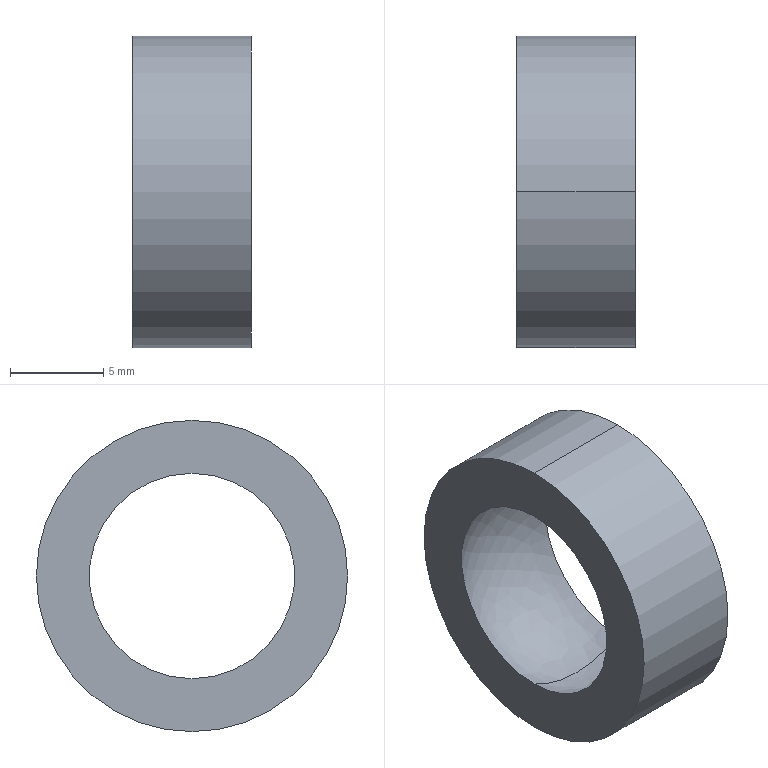Part | SolidWorks | features BaseBody 1 | 1 solid | 6 faces | box 6.35 x 16.667 x 16.667 mm | volume 648.125 mm3 | spline 2 | cylinder 2 | plane 2 | commonest cylinder face diameters 16.667 x2
STEP:
#1=CARTESIAN_POINT('',(3.175,0.,-5.499));
#2=VERTEX_POINT('',#1);
#3=CARTESIAN_POINT('',(3.175,0.,5.499));
#4=VERTEX_POINT('',#3);
#5=CARTESIAN_POINT('',(3.175,0.,0.));
#6=DIRECTION('',(1.,0.,0.));
#7=DIRECTION('',(0.,0.,1.));
#8=AXIS2_PLACEMENT_3D('',#5,#6,#7);
#9=CIRCLE('',#8,5.499);
#10=EDGE_CURVE('',#2,#4,#9,.T.);
#11=ORIENTED_EDGE('',*,*,#10,.T.);
#12=CARTESIAN_POINT('',(-3.175,0.,5.499));
#13=VERTEX_POINT('',#12);
#14=CARTESIAN_POINT('',(0.,0.,0.));
#15=DIRECTION('',(0.,-1.,0.));
#16=DIRECTION('',(1.,0.,0.));
#17=AXIS2_PLACEMENT_3D('',#14,#15,#16);
#18=CIRCLE('',#17,6.35);
#19=EDGE_CURVE('',#4,#13,#18,.T.);
#20=ORIENTED_EDGE('',*,*,#19,.T.);
#21=CARTESIAN_POINT('',(-3.175,0.,-5.499));
#22=VERTEX_POINT('',#21);
#23=CARTESIAN_POINT('',(-3.175,0.,0.));
#24=DIRECTION('',(-1.,0.,0.));
#25=DIRECTION('',(0.,0.,1.));
#26=AXIS2_PLACEMENT_3D('',#23,#24,#25);
#27=CIRCLE('',#26,5.499);
#28=EDGE_CURVE('',#13,#22,#27,.T.);
#29=ORIENTED_EDGE('',*,*,#28,.T.);
#30=CARTESIAN_POINT('',(0.,0.,0.));
#31=DIRECTION('',(0.,1.,0.));
#32=DIRECTION('',(1.,0.,0.));
#33=AXIS2_PLACEMENT_3D('',#30,#31,#32);
#34=CIRCLE('',#33,6.35);
#35=EDGE_CURVE('',#2,#22,#34,.T.);
#36=ORIENTED_EDGE('',*,*,#35,.F.);
#37=EDGE_LOOP('',(#11,#20,#29,#36));
#38=FACE_OUTER_BOUND('',#37,.T.);
#39=CARTESIAN_POINT('',(3.175,0.,5.499));
#40=CARTESIAN_POINT('',(3.175,10.999,5.499));
#41=CARTESIAN_POINT('',(3.175,10.999,-5.499));
#42=CARTESIAN_POINT('',(3.175,0.,-5.499));
#43=CARTESIAN_POINT('',(1.162,0.,6.661));
#44=CARTESIAN_POINT('',(1.162,13.323,6.661));
#45=CARTESIAN_POINT('',(1.162,13.323,-6.661));
#46=CARTESIAN_POINT('',(1.162,0.,-6.661));
#47=CARTESIAN_POINT('',(-1.162,0.,6.661));
#48=CARTESIAN_POINT('',(-1.162,13.323,6.661));
#49=CARTESIAN_POINT('',(-1.162,13.323,-6.661));
#50=CARTESIAN_POINT('',(-1.162,0.,-6.661));
#51=CARTESIAN_POINT('',(-3.175,0.,5.499));
#52=CARTESIAN_POINT('',(-3.175,10.999,5.499));
#53=CARTESIAN_POINT('',(-3.175,10.999,-5.499));
#54=CARTESIAN_POINT('',(-3.175,0.,-5.499));
#55=(BOUNDED_SURFACE()B_SPLINE_SURFACE(3,3,((#39,#40,#41,#42),(#43,#44,#45,#46),(#47,#48,#49,#50),(#51,#52,#53,#54)),.UNSPECIFIED.,.F.,.F.,.T.)B_SPLINE_SURFACE_WITH_KNOTS((4,4),(4,4),(0.,1.),(0.,1.),.UNSPECIFIED.)GEOMETRIC_REPRESENTATION_ITEM()RATIONAL_B_SPLINE_SURFACE(((1.,0.3333,0.3333,1.),(0.9107,0.3036,0.3036,0.9107),(0.9107,0.3036,0.3036,0.9107),(1.,0.3333,0.3333,1.)))REPRESENTATION_ITEM('')SURFACE());
#56=ADVANCED_FACE('',(#38),#55,.T.);
#57=CARTESIAN_POINT('',(3.175,0.,-8.334));
#58=VERTEX_POINT('',#57);
#59=CARTESIAN_POINT('',(3.175,0.,8.334));
#60=VERTEX_POINT('',#59);
#61=CARTESIAN_POINT('',(3.175,0.,0.));
#62=DIRECTION('',(1.,0.,0.));
#63=DIRECTION('',(0.,0.,1.));
#64=AXIS2_PLACEMENT_3D('',#61,#62,#63);
#65=CIRCLE('',#64,8.334);
#66=EDGE_CURVE('',#58,#60,#65,.T.);
#67=ORIENTED_EDGE('',*,*,#66,.F.);
#68=CARTESIAN_POINT('',(-3.175,0.,-8.334));
#69=VERTEX_POINT('',#68);
#70=CARTESIAN_POINT('',(3.175,0.,-8.334));
#71=DIRECTION('',(-1.,0.,0.));
#72=VECTOR('',#71,1000.);
#73=LINE('',#70,#72);
#74=EDGE_CURVE('',#58,#69,#73,.T.);
#75=ORIENTED_EDGE('',*,*,#74,.T.);
#76=CARTESIAN_POINT('',(-3.175,0.,8.334));
#77=VERTEX_POINT('',#76);
#78=CARTESIAN_POINT('',(-3.175,0.,0.));
#79=DIRECTION('',(-1.,0.,0.));
#80=DIRECTION('',(0.,0.,1.));
#81=AXIS2_PLACEMENT_3D('',#78,#79,#80);
#82=CIRCLE('',#81,8.334);
#83=EDGE_CURVE('',#77,#69,#82,.T.);
#84=ORIENTED_EDGE('',*,*,#83,.F.);
#85=CARTESIAN_POINT('',(3.175,0.,8.334));
#86=DIRECTION('',(-1.,0.,0.));
#87=VECTOR('',#86,1000.);
#88=LINE('',#85,#87);
#89=EDGE_CURVE('',#60,#77,#88,.T.);
#90=ORIENTED_EDGE('',*,*,#89,.F.);
#91=EDGE_LOOP('',(#67,#75,#84,#90));
#92=FACE_OUTER_BOUND('',#91,.T.);
#93=CARTESIAN_POINT('',(3.175,0.,0.));
#94=DIRECTION('',(-1.,0.,0.));
#95=DIRECTION('',(0.,0.,1.));
#96=AXIS2_PLACEMENT_3D('',#93,#94,#95);
#97=CYLINDRICAL_SURFACE('',#96,8.334);
#98=ADVANCED_FACE('',(#92),#97,.T.);
#99=ORIENTED_EDGE('',*,*,#19,.F.);
#100=CARTESIAN_POINT('',(3.175,0.,0.));
#101=DIRECTION('',(1.,0.,0.));
#102=DIRECTION('',(0.,0.,1.));
#103=AXIS2_PLACEMENT_3D('',#100,#101,#102);
#104=CIRCLE('',#103,5.499);
#105=EDGE_CURVE('',#4,#2,#104,.T.);
#106=ORIENTED_EDGE('',*,*,#105,.T.);
#107=ORIENTED_EDGE('',*,*,#35,.T.);
#108=CARTESIAN_POINT('',(-3.175,0.,0.));
#109=DIRECTION('',(-1.,0.,0.));
#110=DIRECTION('',(0.,0.,1.));
#111=AXIS2_PLACEMENT_3D('',#108,#109,#110);
#112=CIRCLE('',#111,5.499);
#113=EDGE_CURVE('',#22,#13,#112,.T.);
#114=ORIENTED_EDGE('',*,*,#113,.T.);
#115=EDGE_LOOP('',(#99,#106,#107,#114));
#116=FACE_OUTER_BOUND('',#115,.T.);
#117=CARTESIAN_POINT('',(3.175,0.,-5.499));
#118=CARTESIAN_POINT('',(3.175,-10.999,-5.499));
#119=CARTESIAN_POINT('',(3.175,-10.999,5.499));
#120=CARTESIAN_POINT('',(3.175,0.,5.499));
#121=CARTESIAN_POINT('',(1.162,0.,-6.661));
#122=CARTESIAN_POINT('',(1.162,-13.323,-6.661));
#123=CARTESIAN_POINT('',(1.162,-13.323,6.661));
#124=CARTESIAN_POINT('',(1.162,0.,6.661));
#125=CARTESIAN_POINT('',(-1.162,0.,-6.661));
#126=CARTESIAN_POINT('',(-1.162,-13.323,-6.661));
#127=CARTESIAN_POINT('',(-1.162,-13.323,6.661));
#128=CARTESIAN_POINT('',(-1.162,0.,6.661));
#129=CARTESIAN_POINT('',(-3.175,0.,-5.499));
#130=CARTESIAN_POINT('',(-3.175,-10.999,-5.499));
#131=CARTESIAN_POINT('',(-3.175,-10.999,5.499));
#132=CARTESIAN_POINT('',(-3.175,0.,5.499));
#133=(BOUNDED_SURFACE()B_SPLINE_SURFACE(3,3,((#117,#118,#119,#120),(#121,#122,#123,#124),(#125,#126,#127,#128),(#129,#130,#131,#132)),.UNSPECIFIED.,.F.,.F.,.T.)B_SPLINE_SURFACE_WITH_KNOTS((4,4),(4,4),(0.,1.),(0.,1.),.UNSPECIFIED.)GEOMETRIC_REPRESENTATION_ITEM()RATIONAL_B_SPLINE_SURFACE(((1.,0.3333,0.3333,1.),(0.9107,0.3036,0.3036,0.9107),(0.9107,0.3036,0.3036,0.9107),(1.,0.3333,0.3333,1.)))REPRESENTATION_ITEM('')SURFACE());
#134=ADVANCED_FACE('',(#116),#133,.T.);
#135=ORIENTED_EDGE('',*,*,#113,.F.);
#136=ORIENTED_EDGE('',*,*,#28,.F.);
#137=EDGE_LOOP('',(#135,#136));
#138=FACE_BOUND('',#137,.T.);
#139=ORIENTED_EDGE('',*,*,#83,.T.);
#140=CARTESIAN_POINT('',(-3.175,0.,0.));
#141=DIRECTION('',(-1.,0.,0.));
#142=DIRECTION('',(0.,0.,1.));
#143=AXIS2_PLACEMENT_3D('',#140,#141,#142);
#144=CIRCLE('',#143,8.334);
#145=EDGE_CURVE('',#69,#77,#144,.T.);
#146=ORIENTED_EDGE('',*,*,#145,.T.);
#147=EDGE_LOOP('',(#139,#146));
#148=FACE_OUTER_BOUND('',#147,.T.);
#149=CARTESIAN_POINT('',(-3.175,-8.434,-8.434));
#150=DIRECTION('',(-1.,0.,0.));
#151=DIRECTION('',(0.,0.,1.));
#152=AXIS2_PLACEMENT_3D('',#149,#150,#151);
#153=PLANE('',#152);
#154=ADVANCED_FACE('',(#138,#148),#153,.T.);
#155=ORIENTED_EDGE('',*,*,#10,.F.);
#156=ORIENTED_EDGE('',*,*,#105,.F.);
#157=EDGE_LOOP('',(#155,#156));
#158=FACE_BOUND('',#157,.T.);
#159=CARTESIAN_POINT('',(3.175,0.,0.));
#160=DIRECTION('',(1.,0.,0.));
#161=DIRECTION('',(0.,0.,1.));
#162=AXIS2_PLACEMENT_3D('',#159,#160,#161);
#163=CIRCLE('',#162,8.334);
#164=EDGE_CURVE('',#60,#58,#163,.T.);
#165=ORIENTED_EDGE('',*,*,#164,.T.);
#166=ORIENTED_EDGE('',*,*,#66,.T.);
#167=EDGE_LOOP('',(#165,#166));
#168=FACE_OUTER_BOUND('',#167,.T.);
#169=CARTESIAN_POINT('',(3.175,-8.434,8.434));
#170=DIRECTION('',(1.,0.,0.));
#171=DIRECTION('',(0.,0.,-1.));
#172=AXIS2_PLACEMENT_3D('',#169,#170,#171);
#173=PLANE('',#172);
#174=ADVANCED_FACE('',(#158,#168),#173,.T.);
#175=ORIENTED_EDGE('',*,*,#74,.F.);
#176=ORIENTED_EDGE('',*,*,#164,.F.);
#177=ORIENTED_EDGE('',*,*,#89,.T.);
#178=ORIENTED_EDGE('',*,*,#145,.F.);
#179=EDGE_LOOP('',(#175,#176,#177,#178));
#180=FACE_OUTER_BOUND('',#179,.T.);
#181=CARTESIAN_POINT('',(3.175,0.,0.));
#182=DIRECTION('',(-1.,0.,0.));
#183=DIRECTION('',(0.,0.,1.));
#184=AXIS2_PLACEMENT_3D('',#181,#182,#183);
#185=CYLINDRICAL_SURFACE('',#184,8.334);
#186=ADVANCED_FACE('',(#180),#185,.T.);
#187=CLOSED_SHELL('',(#56,#98,#134,#154,#174,#186));
#188=MANIFOLD_SOLID_BREP('',#187);
#189=CARTESIAN_POINT('',(0.,0.,0.));
#190=DIRECTION('',(0.,0.,1.));
#191=DIRECTION('',(1.,0.,0.));
#192=AXIS2_PLACEMENT_3D('',#189,#190,#191);
#193=(LENGTH_UNIT()NAMED_UNIT(*)SI_UNIT(.MILLI.,.METRE.));
#194=UNCERTAINTY_MEASURE_WITH_UNIT(LENGTH_MEASURE(0.00001),#193,'','');
#195=(NAMED_UNIT(*)PLANE_ANGLE_UNIT()SI_UNIT($,.RADIAN.));
#196=(NAMED_UNIT(*)SI_UNIT($,.STERADIAN.)SOLID_ANGLE_UNIT());
#197=(GEOMETRIC_REPRESENTATION_CONTEXT(3)GLOBAL_UNCERTAINTY_ASSIGNED_CONTEXT((#194))GLOBAL_UNIT_ASSIGNED_CONTEXT((#193,#195,#196))REPRESENTATION_CONTEXT('',''));
#198=ADVANCED_BREP_SHAPE_REPRESENTATION('',(#188,#192),#197);